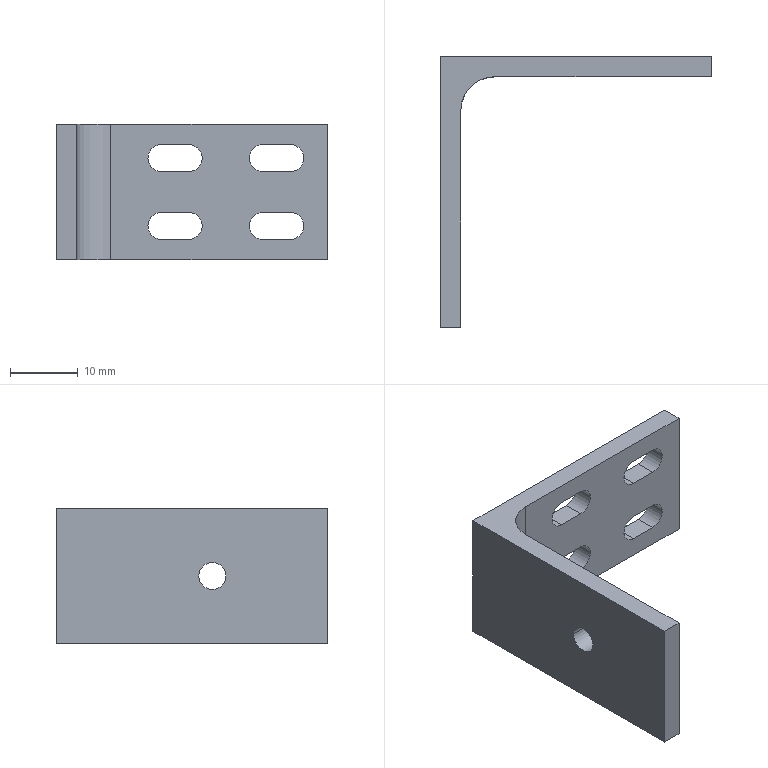Part | STEP file | L40 angle steel | 1 solid | 31 faces | box 40 x 40 x 20 mm | volume 4347 mm3 | plane 16 | cylinder 15 | commonest cylinder face diameters 4 x14 10 x1
STEP:
#1=CARTESIAN_POINT('',(3.,-21.,10.));
#2=VERTEX_POINT('',#1);
#3=CARTESIAN_POINT('',(3.,-25.,10.));
#4=VERTEX_POINT('',#3);
#5=CARTESIAN_POINT('',(3.,-23.,10.));
#6=DIRECTION('',(-1.,0.,0.));
#7=DIRECTION('',(0.,-1.,0.));
#8=AXIS2_PLACEMENT_3D('',#5,#6,#7);
#9=CIRCLE('',#8,2.);
#10=EDGE_CURVE('',#2,#4,#9,.T.);
#11=ORIENTED_EDGE('',*,*,#10,.F.);
#12=CARTESIAN_POINT('',(0.,-21.,10.));
#13=VERTEX_POINT('',#12);
#14=CARTESIAN_POINT('',(20.,-21.,10.));
#15=DIRECTION('',(-1.,0.,0.));
#16=VECTOR('',#15,1000.);
#17=LINE('',#14,#16);
#18=EDGE_CURVE('',#2,#13,#17,.T.);
#19=ORIENTED_EDGE('',*,*,#18,.T.);
#20=CARTESIAN_POINT('',(0.,-25.,10.));
#21=VERTEX_POINT('',#20);
#22=CARTESIAN_POINT('',(0.,-23.,10.));
#23=DIRECTION('',(-1.,0.,0.));
#24=DIRECTION('',(0.,-1.,0.));
#25=AXIS2_PLACEMENT_3D('',#22,#23,#24);
#26=CIRCLE('',#25,2.);
#27=EDGE_CURVE('',#13,#21,#26,.T.);
#28=ORIENTED_EDGE('',*,*,#27,.T.);
#29=CARTESIAN_POINT('',(20.,-25.,10.));
#30=DIRECTION('',(-1.,0.,0.));
#31=VECTOR('',#30,1000.);
#32=LINE('',#29,#31);
#33=EDGE_CURVE('',#4,#21,#32,.T.);
#34=ORIENTED_EDGE('',*,*,#33,.F.);
#35=EDGE_LOOP('',(#11,#19,#28,#34));
#36=FACE_OUTER_BOUND('',#35,.T.);
#37=CARTESIAN_POINT('',(20.,-23.,10.));
#38=DIRECTION('',(-1.,0.,0.));
#39=DIRECTION('',(0.,-1.,0.));
#40=AXIS2_PLACEMENT_3D('',#37,#38,#39);
#41=CYLINDRICAL_SURFACE('',#40,2.);
#42=ADVANCED_FACE('',(#36),#41,.F.);
#43=CARTESIAN_POINT('',(30.5,-3.,7.));
#44=VERTEX_POINT('',#43);
#45=CARTESIAN_POINT('',(28.5,-3.,5.));
#46=VERTEX_POINT('',#45);
#47=CARTESIAN_POINT('',(30.5,-3.,5.));
#48=DIRECTION('',(0.,-1.,0.));
#49=DIRECTION('',(-1.,0.,0.));
#50=AXIS2_PLACEMENT_3D('',#47,#48,#49);
#51=CIRCLE('',#50,2.);
#52=EDGE_CURVE('',#44,#46,#51,.T.);
#53=ORIENTED_EDGE('',*,*,#52,.T.);
#54=CARTESIAN_POINT('',(28.5,0.,5.));
#55=VERTEX_POINT('',#54);
#56=CARTESIAN_POINT('',(28.5,-20.,5.));
#57=DIRECTION('',(0.,1.,0.));
#58=VECTOR('',#57,1000.);
#59=LINE('',#56,#58);
#60=EDGE_CURVE('',#46,#55,#59,.T.);
#61=ORIENTED_EDGE('',*,*,#60,.T.);
#62=CARTESIAN_POINT('',(30.5,0.,7.));
#63=VERTEX_POINT('',#62);
#64=CARTESIAN_POINT('',(30.5,0.,5.));
#65=DIRECTION('',(0.,1.,0.));
#66=DIRECTION('',(-1.,0.,0.));
#67=AXIS2_PLACEMENT_3D('',#64,#65,#66);
#68=CIRCLE('',#67,2.);
#69=EDGE_CURVE('',#55,#63,#68,.T.);
#70=ORIENTED_EDGE('',*,*,#69,.T.);
#71=CARTESIAN_POINT('',(30.5,-20.,7.));
#72=DIRECTION('',(0.,-1.,0.));
#73=VECTOR('',#72,1000.);
#74=LINE('',#71,#73);
#75=EDGE_CURVE('',#63,#44,#74,.T.);
#76=ORIENTED_EDGE('',*,*,#75,.T.);
#77=EDGE_LOOP('',(#53,#61,#70,#76));
#78=FACE_OUTER_BOUND('',#77,.T.);
#79=CARTESIAN_POINT('',(30.5,-20.,5.));
#80=DIRECTION('',(0.,1.,0.));
#81=DIRECTION('',(-1.,0.,0.));
#82=AXIS2_PLACEMENT_3D('',#79,#80,#81);
#83=CYLINDRICAL_SURFACE('',#82,2.);
#84=ADVANCED_FACE('',(#78),#83,.F.);
#85=CARTESIAN_POINT('',(15.5,-3.,7.));
#86=VERTEX_POINT('',#85);
#87=CARTESIAN_POINT('',(13.5,-3.,5.));
#88=VERTEX_POINT('',#87);
#89=CARTESIAN_POINT('',(15.5,-3.,5.));
#90=DIRECTION('',(0.,-1.,0.));
#91=DIRECTION('',(-1.,0.,0.));
#92=AXIS2_PLACEMENT_3D('',#89,#90,#91);
#93=CIRCLE('',#92,2.);
#94=EDGE_CURVE('',#86,#88,#93,.T.);
#95=ORIENTED_EDGE('',*,*,#94,.T.);
#96=CARTESIAN_POINT('',(13.5,0.,5.));
#97=VERTEX_POINT('',#96);
#98=CARTESIAN_POINT('',(13.5,-20.,5.));
#99=DIRECTION('',(0.,1.,0.));
#100=VECTOR('',#99,1000.);
#101=LINE('',#98,#100);
#102=EDGE_CURVE('',#88,#97,#101,.T.);
#103=ORIENTED_EDGE('',*,*,#102,.T.);
#104=CARTESIAN_POINT('',(15.5,0.,7.));
#105=VERTEX_POINT('',#104);
#106=CARTESIAN_POINT('',(15.5,0.,5.));
#107=DIRECTION('',(0.,1.,0.));
#108=DIRECTION('',(-1.,0.,0.));
#109=AXIS2_PLACEMENT_3D('',#106,#107,#108);
#110=CIRCLE('',#109,2.);
#111=EDGE_CURVE('',#97,#105,#110,.T.);
#112=ORIENTED_EDGE('',*,*,#111,.T.);
#113=CARTESIAN_POINT('',(15.5,-20.,7.));
#114=DIRECTION('',(0.,-1.,0.));
#115=VECTOR('',#114,1000.);
#116=LINE('',#113,#115);
#117=EDGE_CURVE('',#105,#86,#116,.T.);
#118=ORIENTED_EDGE('',*,*,#117,.T.);
#119=EDGE_LOOP('',(#95,#103,#112,#118));
#120=FACE_OUTER_BOUND('',#119,.T.);
#121=CARTESIAN_POINT('',(15.5,-20.,5.));
#122=DIRECTION('',(0.,1.,0.));
#123=DIRECTION('',(-1.,0.,0.));
#124=AXIS2_PLACEMENT_3D('',#121,#122,#123);
#125=CYLINDRICAL_SURFACE('',#124,2.);
#126=ADVANCED_FACE('',(#120),#125,.F.);
#127=CARTESIAN_POINT('',(15.5,-3.,17.));
#128=VERTEX_POINT('',#127);
#129=CARTESIAN_POINT('',(13.5,-3.,15.));
#130=VERTEX_POINT('',#129);
#131=CARTESIAN_POINT('',(15.5,-3.,15.));
#132=DIRECTION('',(0.,-1.,0.));
#133=DIRECTION('',(-1.,0.,0.));
#134=AXIS2_PLACEMENT_3D('',#131,#132,#133);
#135=CIRCLE('',#134,2.);
#136=EDGE_CURVE('',#128,#130,#135,.T.);
#137=ORIENTED_EDGE('',*,*,#136,.T.);
#138=CARTESIAN_POINT('',(13.5,0.,15.));
#139=VERTEX_POINT('',#138);
#140=CARTESIAN_POINT('',(13.5,-20.,15.));
#141=DIRECTION('',(0.,1.,0.));
#142=VECTOR('',#141,1000.);
#143=LINE('',#140,#142);
#144=EDGE_CURVE('',#130,#139,#143,.T.);
#145=ORIENTED_EDGE('',*,*,#144,.T.);
#146=CARTESIAN_POINT('',(15.5,0.,17.));
#147=VERTEX_POINT('',#146);
#148=CARTESIAN_POINT('',(15.5,0.,15.));
#149=DIRECTION('',(0.,1.,0.));
#150=DIRECTION('',(-1.,0.,0.));
#151=AXIS2_PLACEMENT_3D('',#148,#149,#150);
#152=CIRCLE('',#151,2.);
#153=EDGE_CURVE('',#139,#147,#152,.T.);
#154=ORIENTED_EDGE('',*,*,#153,.T.);
#155=CARTESIAN_POINT('',(15.5,-20.,17.));
#156=DIRECTION('',(0.,-1.,0.));
#157=VECTOR('',#156,1000.);
#158=LINE('',#155,#157);
#159=EDGE_CURVE('',#147,#128,#158,.T.);
#160=ORIENTED_EDGE('',*,*,#159,.T.);
#161=EDGE_LOOP('',(#137,#145,#154,#160));
#162=FACE_OUTER_BOUND('',#161,.T.);
#163=CARTESIAN_POINT('',(15.5,-20.,15.));
#164=DIRECTION('',(0.,1.,0.));
#165=DIRECTION('',(-1.,0.,0.));
#166=AXIS2_PLACEMENT_3D('',#163,#164,#165);
#167=CYLINDRICAL_SURFACE('',#166,2.);
#168=ADVANCED_FACE('',(#162),#167,.F.);
#169=CARTESIAN_POINT('',(30.5,-3.,17.));
#170=VERTEX_POINT('',#169);
#171=CARTESIAN_POINT('',(28.5,-3.,15.));
#172=VERTEX_POINT('',#171);
#173=CARTESIAN_POINT('',(30.5,-3.,15.));
#174=DIRECTION('',(0.,-1.,0.));
#175=DIRECTION('',(-1.,0.,0.));
#176=AXIS2_PLACEMENT_3D('',#173,#174,#175);
#177=CIRCLE('',#176,2.);
#178=EDGE_CURVE('',#170,#172,#177,.T.);
#179=ORIENTED_EDGE('',*,*,#178,.T.);
#180=CARTESIAN_POINT('',(28.5,0.,15.));
#181=VERTEX_POINT('',#180);
#182=CARTESIAN_POINT('',(28.5,-20.,15.));
#183=DIRECTION('',(0.,1.,0.));
#184=VECTOR('',#183,1000.);
#185=LINE('',#182,#184);
#186=EDGE_CURVE('',#172,#181,#185,.T.);
#187=ORIENTED_EDGE('',*,*,#186,.T.);
#188=CARTESIAN_POINT('',(30.5,0.,17.));
#189=VERTEX_POINT('',#188);
#190=CARTESIAN_POINT('',(30.5,0.,15.));
#191=DIRECTION('',(0.,1.,0.));
#192=DIRECTION('',(-1.,0.,0.));
#193=AXIS2_PLACEMENT_3D('',#190,#191,#192);
#194=CIRCLE('',#193,2.);
#195=EDGE_CURVE('',#181,#189,#194,.T.);
#196=ORIENTED_EDGE('',*,*,#195,.T.);
#197=CARTESIAN_POINT('',(30.5,-20.,17.));
#198=DIRECTION('',(0.,-1.,0.));
#199=VECTOR('',#198,1000.);
#200=LINE('',#197,#199);
#201=EDGE_CURVE('',#189,#170,#200,.T.);
#202=ORIENTED_EDGE('',*,*,#201,.T.);
#203=EDGE_LOOP('',(#179,#187,#196,#202));
#204=FACE_OUTER_BOUND('',#203,.T.);
#205=CARTESIAN_POINT('',(30.5,-20.,15.));
#206=DIRECTION('',(0.,1.,0.));
#207=DIRECTION('',(-1.,0.,0.));
#208=AXIS2_PLACEMENT_3D('',#205,#206,#207);
#209=CYLINDRICAL_SURFACE('',#208,2.);
#210=ADVANCED_FACE('',(#204),#209,.F.);
#211=CARTESIAN_POINT('',(0.,-40.,20.));
#212=VERTEX_POINT('',#211);
#213=CARTESIAN_POINT('',(0.,-40.,0.));
#214=VERTEX_POINT('',#213);
#215=CARTESIAN_POINT('',(0.,-40.,20.));
#216=DIRECTION('',(0.,0.,-1.));
#217=VECTOR('',#216,1000.);
#218=LINE('',#215,#217);
#219=EDGE_CURVE('',#212,#214,#218,.T.);
#220=ORIENTED_EDGE('',*,*,#219,.F.);
#221=CARTESIAN_POINT('',(0.,0.,20.));
#222=VERTEX_POINT('',#221);
#223=CARTESIAN_POINT('',(0.,0.,20.));
#224=DIRECTION('',(0.,-1.,0.));
#225=VECTOR('',#224,1000.);
#226=LINE('',#223,#225);
#227=EDGE_CURVE('',#222,#212,#226,.T.);
#228=ORIENTED_EDGE('',*,*,#227,.F.);
#229=CARTESIAN_POINT('',(0.,0.,0.));
#230=VERTEX_POINT('',#229);
#231=CARTESIAN_POINT('',(0.,0.,20.));
#232=DIRECTION('',(0.,0.,1.));
#233=VECTOR('',#232,1000.);
#234=LINE('',#231,#233);
#235=EDGE_CURVE('',#230,#222,#234,.T.);
#236=ORIENTED_EDGE('',*,*,#235,.F.);
#237=CARTESIAN_POINT('',(0.,0.,0.));
#238=DIRECTION('',(0.,1.,0.));
#239=VECTOR('',#238,1000.);
#240=LINE('',#237,#239);
#241=EDGE_CURVE('',#214,#230,#240,.T.);
#242=ORIENTED_EDGE('',*,*,#241,.F.);
#243=EDGE_LOOP('',(#220,#228,#236,#242));
#244=FACE_OUTER_BOUND('',#243,.T.);
#245=CARTESIAN_POINT('',(0.,-23.,10.));
#246=DIRECTION('',(-1.,0.,0.));
#247=DIRECTION('',(0.,-1.,0.));
#248=AXIS2_PLACEMENT_3D('',#245,#246,#247);
#249=CIRCLE('',#248,2.);
#250=EDGE_CURVE('',#21,#13,#249,.T.);
#251=ORIENTED_EDGE('',*,*,#250,.F.);
#252=ORIENTED_EDGE('',*,*,#27,.F.);
#253=EDGE_LOOP('',(#251,#252));
#254=FACE_BOUND('',#253,.T.);
#255=CARTESIAN_POINT('',(0.,0.,20.));
#256=DIRECTION('',(1.,0.,0.));
#257=DIRECTION('',(0.,1.,0.));
#258=AXIS2_PLACEMENT_3D('',#255,#256,#257);
#259=PLANE('',#258);
#260=ADVANCED_FACE('',(#244,#254),#259,.F.);
#261=ORIENTED_EDGE('',*,*,#241,.T.);
#262=CARTESIAN_POINT('',(40.,0.,0.));
#263=VERTEX_POINT('',#262);
#264=CARTESIAN_POINT('',(8.,0.,0.));
#265=DIRECTION('',(1.,0.,0.));
#266=VECTOR('',#265,1000.);
#267=LINE('',#264,#266);
#268=EDGE_CURVE('',#230,#263,#267,.T.);
#269=ORIENTED_EDGE('',*,*,#268,.T.);
#270=CARTESIAN_POINT('',(40.,-3.,0.));
#271=VERTEX_POINT('',#270);
#272=CARTESIAN_POINT('',(40.,-8.,0.));
#273=DIRECTION('',(0.,-1.,0.));
#274=VECTOR('',#273,1000.);
#275=LINE('',#272,#274);
#276=EDGE_CURVE('',#263,#271,#275,.T.);
#277=ORIENTED_EDGE('',*,*,#276,.T.);
#278=CARTESIAN_POINT('',(8.,-3.,0.));
#279=VERTEX_POINT('',#278);
#280=CARTESIAN_POINT('',(8.,-3.,0.));
#281=DIRECTION('',(-1.,0.,0.));
#282=VECTOR('',#281,1000.);
#283=LINE('',#280,#282);
#284=EDGE_CURVE('',#271,#279,#283,.T.);
#285=ORIENTED_EDGE('',*,*,#284,.T.);
#286=CARTESIAN_POINT('',(3.,-8.,0.));
#287=VERTEX_POINT('',#286);
#288=CARTESIAN_POINT('',(8.,-8.,0.));
#289=DIRECTION('',(0.,0.,1.));
#290=DIRECTION('',(-1.,0.,0.));
#291=AXIS2_PLACEMENT_3D('',#288,#289,#290);
#292=CIRCLE('',#291,5.);
#293=EDGE_CURVE('',#279,#287,#292,.T.);
#294=ORIENTED_EDGE('',*,*,#293,.T.);
#295=CARTESIAN_POINT('',(3.,-40.,0.));
#296=VERTEX_POINT('',#295);
#297=CARTESIAN_POINT('',(3.,-8.,0.));
#298=DIRECTION('',(0.,-1.,0.));
#299=VECTOR('',#298,1000.);
#300=LINE('',#297,#299);
#301=EDGE_CURVE('',#287,#296,#300,.T.);
#302=ORIENTED_EDGE('',*,*,#301,.T.);
#303=CARTESIAN_POINT('',(8.,-40.,0.));
#304=DIRECTION('',(-1.,0.,0.));
#305=VECTOR('',#304,1000.);
#306=LINE('',#303,#305);
#307=EDGE_CURVE('',#296,#214,#306,.T.);
#308=ORIENTED_EDGE('',*,*,#307,.T.);
#309=EDGE_LOOP('',(#261,#269,#277,#285,#294,#302,#308));
#310=FACE_OUTER_BOUND('',#309,.T.);
#311=CARTESIAN_POINT('',(8.,-8.,0.));
#312=DIRECTION('',(0.,0.,-1.));
#313=DIRECTION('',(-1.,0.,0.));
#314=AXIS2_PLACEMENT_3D('',#311,#312,#313);
#315=PLANE('',#314);
#316=ADVANCED_FACE('',(#310),#315,.T.);
#317=CARTESIAN_POINT('',(3.,-40.,20.));
#318=VERTEX_POINT('',#317);
#319=CARTESIAN_POINT('',(3.,-40.,20.));
#320=DIRECTION('',(0.,0.,-1.));
#321=VECTOR('',#320,1000.);
#322=LINE('',#319,#321);
#323=EDGE_CURVE('',#318,#296,#322,.T.);
#324=ORIENTED_EDGE('',*,*,#323,.F.);
#325=CARTESIAN_POINT('',(3.,-40.,20.));
#326=DIRECTION('',(1.,0.,0.));
#327=VECTOR('',#326,1000.);
#328=LINE('',#325,#327);
#329=EDGE_CURVE('',#212,#318,#328,.T.);
#330=ORIENTED_EDGE('',*,*,#329,.F.);
#331=ORIENTED_EDGE('',*,*,#219,.T.);
#332=ORIENTED_EDGE('',*,*,#307,.F.);
#333=EDGE_LOOP('',(#324,#330,#331,#332));
#334=FACE_OUTER_BOUND('',#333,.T.);
#335=CARTESIAN_POINT('',(3.,-40.,20.));
#336=DIRECTION('',(0.,1.,0.));
#337=DIRECTION('',(0.,0.,1.));
#338=AXIS2_PLACEMENT_3D('',#335,#336,#337);
#339=PLANE('',#338);
#340=ADVANCED_FACE('',(#334),#339,.F.);
#341=CARTESIAN_POINT('',(40.,0.,20.));
#342=VERTEX_POINT('',#341);
#343=CARTESIAN_POINT('',(8.,0.,20.));
#344=DIRECTION('',(1.,0.,0.));
#345=VECTOR('',#344,1000.);
#346=LINE('',#343,#345);
#347=EDGE_CURVE('',#222,#342,#346,.T.);
#348=ORIENTED_EDGE('',*,*,#347,.F.);
#349=ORIENTED_EDGE('',*,*,#227,.T.);
#350=ORIENTED_EDGE('',*,*,#329,.T.);
#351=CARTESIAN_POINT('',(3.,-8.,20.));
#352=VERTEX_POINT('',#351);
#353=CARTESIAN_POINT('',(3.,-8.,20.));
#354=DIRECTION('',(0.,-1.,0.));
#355=VECTOR('',#354,1000.);
#356=LINE('',#353,#355);
#357=EDGE_CURVE('',#352,#318,#356,.T.);
#358=ORIENTED_EDGE('',*,*,#357,.F.);
#359=CARTESIAN_POINT('',(8.,-3.,20.));
#360=VERTEX_POINT('',#359);
#361=CARTESIAN_POINT('',(8.,-8.,20.));
#362=DIRECTION('',(0.,0.,1.));
#363=DIRECTION('',(-1.,0.,0.));
#364=AXIS2_PLACEMENT_3D('',#361,#362,#363);
#365=CIRCLE('',#364,5.);
#366=EDGE_CURVE('',#360,#352,#365,.T.);
#367=ORIENTED_EDGE('',*,*,#366,.F.);
#368=CARTESIAN_POINT('',(40.,-3.,20.));
#369=VERTEX_POINT('',#368);
#370=CARTESIAN_POINT('',(8.,-3.,20.));
#371=DIRECTION('',(-1.,0.,0.));
#372=VECTOR('',#371,1000.);
#373=LINE('',#370,#372);
#374=EDGE_CURVE('',#369,#360,#373,.T.);
#375=ORIENTED_EDGE('',*,*,#374,.F.);
#376=CARTESIAN_POINT('',(40.,-8.,20.));
#377=DIRECTION('',(0.,-1.,0.));
#378=VECTOR('',#377,1000.);
#379=LINE('',#376,#378);
#380=EDGE_CURVE('',#342,#369,#379,.T.);
#381=ORIENTED_EDGE('',*,*,#380,.F.);
#382=EDGE_LOOP('',(#348,#349,#350,#358,#367,#375,#381));
#383=FACE_OUTER_BOUND('',#382,.T.);
#384=CARTESIAN_POINT('',(8.,-8.,20.));
#385=DIRECTION('',(0.,0.,-1.));
#386=DIRECTION('',(-1.,0.,0.));
#387=AXIS2_PLACEMENT_3D('',#384,#385,#386);
#388=PLANE('',#387);
#389=ADVANCED_FACE('',(#383),#388,.F.);
#390=ORIENTED_EDGE('',*,*,#235,.T.);
#391=ORIENTED_EDGE('',*,*,#347,.T.);
#392=CARTESIAN_POINT('',(40.,0.,20.));
#393=DIRECTION('',(0.,0.,1.));
#394=VECTOR('',#393,1000.);
#395=LINE('',#392,#394);
#396=EDGE_CURVE('',#263,#342,#395,.T.);
#397=ORIENTED_EDGE('',*,*,#396,.F.);
#398=ORIENTED_EDGE('',*,*,#268,.F.);
#399=EDGE_LOOP('',(#390,#391,#397,#398));
#400=FACE_OUTER_BOUND('',#399,.T.);
#401=CARTESIAN_POINT('',(30.5,0.,3.));
#402=VERTEX_POINT('',#401);
#403=CARTESIAN_POINT('',(30.5,0.,5.));
#404=DIRECTION('',(0.,1.,0.));
#405=DIRECTION('',(-1.,0.,0.));
#406=AXIS2_PLACEMENT_3D('',#403,#404,#405);
#407=CIRCLE('',#406,2.);
#408=EDGE_CURVE('',#402,#55,#407,.T.);
#409=ORIENTED_EDGE('',*,*,#408,.F.);
#410=CARTESIAN_POINT('',(34.5,0.,3.));
#411=VERTEX_POINT('',#410);
#412=CARTESIAN_POINT('',(40.,0.,3.));
#413=DIRECTION('',(-1.,0.,0.));
#414=VECTOR('',#413,1000.);
#415=LINE('',#412,#414);
#416=EDGE_CURVE('',#411,#402,#415,.T.);
#417=ORIENTED_EDGE('',*,*,#416,.F.);
#418=CARTESIAN_POINT('',(34.5,0.,7.));
#419=VERTEX_POINT('',#418);
#420=CARTESIAN_POINT('',(34.5,0.,5.));
#421=DIRECTION('',(0.,1.,0.));
#422=DIRECTION('',(-1.,0.,0.));
#423=AXIS2_PLACEMENT_3D('',#420,#421,#422);
#424=CIRCLE('',#423,2.);
#425=EDGE_CURVE('',#419,#411,#424,.T.);
#426=ORIENTED_EDGE('',*,*,#425,.F.);
#427=CARTESIAN_POINT('',(40.,0.,7.));
#428=DIRECTION('',(1.,0.,0.));
#429=VECTOR('',#428,1000.);
#430=LINE('',#427,#429);
#431=EDGE_CURVE('',#63,#419,#430,.T.);
#432=ORIENTED_EDGE('',*,*,#431,.F.);
#433=ORIENTED_EDGE('',*,*,#69,.F.);
#434=EDGE_LOOP('',(#409,#417,#426,#432,#433));
#435=FACE_BOUND('',#434,.T.);
#436=CARTESIAN_POINT('',(15.5,0.,3.));
#437=VERTEX_POINT('',#436);
#438=CARTESIAN_POINT('',(15.5,0.,5.));
#439=DIRECTION('',(0.,1.,0.));
#440=DIRECTION('',(-1.,0.,0.));
#441=AXIS2_PLACEMENT_3D('',#438,#439,#440);
#442=CIRCLE('',#441,2.);
#443=EDGE_CURVE('',#437,#97,#442,.T.);
#444=ORIENTED_EDGE('',*,*,#443,.F.);
#445=CARTESIAN_POINT('',(19.5,0.,3.));
#446=VERTEX_POINT('',#445);
#447=CARTESIAN_POINT('',(40.,0.,3.));
#448=DIRECTION('',(-1.,0.,0.));
#449=VECTOR('',#448,1000.);
#450=LINE('',#447,#449);
#451=EDGE_CURVE('',#446,#437,#450,.T.);
#452=ORIENTED_EDGE('',*,*,#451,.F.);
#453=CARTESIAN_POINT('',(19.5,0.,7.));
#454=VERTEX_POINT('',#453);
#455=CARTESIAN_POINT('',(19.5,0.,5.));
#456=DIRECTION('',(0.,1.,0.));
#457=DIRECTION('',(-1.,0.,0.));
#458=AXIS2_PLACEMENT_3D('',#455,#456,#457);
#459=CIRCLE('',#458,2.);
#460=EDGE_CURVE('',#454,#446,#459,.T.);
#461=ORIENTED_EDGE('',*,*,#460,.F.);
#462=CARTESIAN_POINT('',(40.,0.,7.));
#463=DIRECTION('',(1.,0.,0.));
#464=VECTOR('',#463,1000.);
#465=LINE('',#462,#464);
#466=EDGE_CURVE('',#105,#454,#465,.T.);
#467=ORIENTED_EDGE('',*,*,#466,.F.);
#468=ORIENTED_EDGE('',*,*,#111,.F.);
#469=EDGE_LOOP('',(#444,#452,#461,#467,#468));
#470=FACE_BOUND('',#469,.T.);
#471=CARTESIAN_POINT('',(15.5,0.,13.));
#472=VERTEX_POINT('',#471);
#473=CARTESIAN_POINT('',(15.5,0.,15.));
#474=DIRECTION('',(0.,1.,0.));
#475=DIRECTION('',(-1.,0.,0.));
#476=AXIS2_PLACEMENT_3D('',#473,#474,#475);
#477=CIRCLE('',#476,2.);
#478=EDGE_CURVE('',#472,#139,#477,.T.);
#479=ORIENTED_EDGE('',*,*,#478,.F.);
#480=CARTESIAN_POINT('',(19.5,0.,13.));
#481=VERTEX_POINT('',#480);
#482=CARTESIAN_POINT('',(40.,0.,13.));
#483=DIRECTION('',(-1.,0.,0.));
#484=VECTOR('',#483,1000.);
#485=LINE('',#482,#484);
#486=EDGE_CURVE('',#481,#472,#485,.T.);
#487=ORIENTED_EDGE('',*,*,#486,.F.);
#488=CARTESIAN_POINT('',(19.5,0.,17.));
#489=VERTEX_POINT('',#488);
#490=CARTESIAN_POINT('',(19.5,0.,15.));
#491=DIRECTION('',(0.,1.,0.));
#492=DIRECTION('',(-1.,0.,0.));
#493=AXIS2_PLACEMENT_3D('',#490,#491,#492);
#494=CIRCLE('',#493,2.);
#495=EDGE_CURVE('',#489,#481,#494,.T.);
#496=ORIENTED_EDGE('',*,*,#495,.F.);
#497=CARTESIAN_POINT('',(40.,0.,17.));
#498=DIRECTION('',(1.,0.,0.));
#499=VECTOR('',#498,1000.);
#500=LINE('',#497,#499);
#501=EDGE_CURVE('',#147,#489,#500,.T.);
#502=ORIENTED_EDGE('',*,*,#501,.F.);
#503=ORIENTED_EDGE('',*,*,#153,.F.);
#504=EDGE_LOOP('',(#479,#487,#496,#502,#503));
#505=FACE_BOUND('',#504,.T.);
#506=CARTESIAN_POINT('',(30.5,0.,13.));
#507=VERTEX_POINT('',#506);
#508=CARTESIAN_POINT('',(30.5,0.,15.));
#509=DIRECTION('',(0.,1.,0.));
#510=DIRECTION('',(-1.,0.,0.));
#511=AXIS2_PLACEMENT_3D('',#508,#509,#510);
#512=CIRCLE('',#511,2.);
#513=EDGE_CURVE('',#507,#181,#512,.T.);
#514=ORIENTED_EDGE('',*,*,#513,.F.);
#515=CARTESIAN_POINT('',(34.5,0.,13.));
#516=VERTEX_POINT('',#515);
#517=CARTESIAN_POINT('',(40.,0.,13.));
#518=DIRECTION('',(-1.,0.,0.));
#519=VECTOR('',#518,1000.);
#520=LINE('',#517,#519);
#521=EDGE_CURVE('',#516,#507,#520,.T.);
#522=ORIENTED_EDGE('',*,*,#521,.F.);
#523=CARTESIAN_POINT('',(34.5,0.,17.));
#524=VERTEX_POINT('',#523);
#525=CARTESIAN_POINT('',(34.5,0.,15.));
#526=DIRECTION('',(0.,1.,0.));
#527=DIRECTION('',(-1.,0.,0.));
#528=AXIS2_PLACEMENT_3D('',#525,#526,#527);
#529=CIRCLE('',#528,2.);
#530=EDGE_CURVE('',#524,#516,#529,.T.);
#531=ORIENTED_EDGE('',*,*,#530,.F.);
#532=CARTESIAN_POINT('',(40.,0.,17.));
#533=DIRECTION('',(1.,0.,0.));
#534=VECTOR('',#533,1000.);
#535=LINE('',#532,#534);
#536=EDGE_CURVE('',#189,#524,#535,.T.);
#537=ORIENTED_EDGE('',*,*,#536,.F.);
#538=ORIENTED_EDGE('',*,*,#195,.F.);
#539=EDGE_LOOP('',(#514,#522,#531,#537,#538));
#540=FACE_BOUND('',#539,.T.);
#541=CARTESIAN_POINT('',(40.,0.,20.));
#542=DIRECTION('',(0.,-1.,0.));
#543=DIRECTION('',(1.,0.,0.));
#544=AXIS2_PLACEMENT_3D('',#541,#542,#543);
#545=PLANE('',#544);
#546=ADVANCED_FACE('',(#400,#435,#470,#505,#540),#545,.F.);
#547=ORIENTED_EDGE('',*,*,#18,.F.);
#548=CARTESIAN_POINT('',(3.,-23.,10.));
#549=DIRECTION('',(-1.,0.,0.));
#550=DIRECTION('',(0.,-1.,0.));
#551=AXIS2_PLACEMENT_3D('',#548,#549,#550);
#552=CIRCLE('',#551,2.);
#553=EDGE_CURVE('',#4,#2,#552,.T.);
#554=ORIENTED_EDGE('',*,*,#553,.F.);
#555=ORIENTED_EDGE('',*,*,#33,.T.);
#556=ORIENTED_EDGE('',*,*,#250,.T.);
#557=EDGE_LOOP('',(#547,#554,#555,#556));
#558=FACE_OUTER_BOUND('',#557,.T.);
#559=CARTESIAN_POINT('',(20.,-23.,10.));
#560=DIRECTION('',(-1.,0.,0.));
#561=DIRECTION('',(0.,-1.,0.));
#562=AXIS2_PLACEMENT_3D('',#559,#560,#561);
#563=CYLINDRICAL_SURFACE('',#562,2.);
#564=ADVANCED_FACE('',(#558),#563,.F.);
#565=CARTESIAN_POINT('',(3.,-8.,20.));
#566=DIRECTION('',(0.,0.,-1.));
#567=VECTOR('',#566,1000.);
#568=LINE('',#565,#567);
#569=EDGE_CURVE('',#352,#287,#568,.T.);
#570=ORIENTED_EDGE('',*,*,#569,.F.);
#571=ORIENTED_EDGE('',*,*,#357,.T.);
#572=ORIENTED_EDGE('',*,*,#323,.T.);
#573=ORIENTED_EDGE('',*,*,#301,.F.);
#574=EDGE_LOOP('',(#570,#571,#572,#573));
#575=FACE_OUTER_BOUND('',#574,.T.);
#576=ORIENTED_EDGE('',*,*,#553,.T.);
#577=ORIENTED_EDGE('',*,*,#10,.T.);
#578=EDGE_LOOP('',(#576,#577));
#579=FACE_BOUND('',#578,.T.);
#580=CARTESIAN_POINT('',(3.,-8.,20.));
#581=DIRECTION('',(-1.,0.,0.));
#582=DIRECTION('',(0.,-1.,0.));
#583=AXIS2_PLACEMENT_3D('',#580,#581,#582);
#584=PLANE('',#583);
#585=ADVANCED_FACE('',(#575,#579),#584,.F.);
#586=CARTESIAN_POINT('',(8.,-3.,20.));
#587=DIRECTION('',(0.,0.,-1.));
#588=VECTOR('',#587,1000.);
#589=LINE('',#586,#588);
#590=EDGE_CURVE('',#360,#279,#589,.T.);
#591=ORIENTED_EDGE('',*,*,#590,.F.);
#592=ORIENTED_EDGE('',*,*,#366,.T.);
#593=ORIENTED_EDGE('',*,*,#569,.T.);
#594=ORIENTED_EDGE('',*,*,#293,.F.);
#595=EDGE_LOOP('',(#591,#592,#593,#594));
#596=FACE_OUTER_BOUND('',#595,.T.);
#597=CARTESIAN_POINT('',(8.,-8.,20.));
#598=DIRECTION('',(0.,0.,-1.));
#599=DIRECTION('',(-1.,0.,0.));
#600=AXIS2_PLACEMENT_3D('',#597,#598,#599);
#601=CYLINDRICAL_SURFACE('',#600,5.);
#602=ADVANCED_FACE('',(#596),#601,.F.);
#603=CARTESIAN_POINT('',(40.,-3.,20.));
#604=DIRECTION('',(0.,0.,-1.));
#605=VECTOR('',#604,1000.);
#606=LINE('',#603,#605);
#607=EDGE_CURVE('',#369,#271,#606,.T.);
#608=ORIENTED_EDGE('',*,*,#607,.F.);
#609=ORIENTED_EDGE('',*,*,#374,.T.);
#610=ORIENTED_EDGE('',*,*,#590,.T.);
#611=ORIENTED_EDGE('',*,*,#284,.F.);
#612=EDGE_LOOP('',(#608,#609,#610,#611));
#613=FACE_OUTER_BOUND('',#612,.T.);
#614=ORIENTED_EDGE('',*,*,#52,.F.);
#615=CARTESIAN_POINT('',(34.5,-3.,7.));
#616=VERTEX_POINT('',#615);
#617=CARTESIAN_POINT('',(40.,-3.,7.));
#618=DIRECTION('',(-1.,0.,0.));
#619=VECTOR('',#618,1000.);
#620=LINE('',#617,#619);
#621=EDGE_CURVE('',#616,#44,#620,.T.);
#622=ORIENTED_EDGE('',*,*,#621,.F.);
#623=CARTESIAN_POINT('',(34.5,-3.,3.));
#624=VERTEX_POINT('',#623);
#625=CARTESIAN_POINT('',(34.5,-3.,5.));
#626=DIRECTION('',(0.,-1.,0.));
#627=DIRECTION('',(-1.,0.,0.));
#628=AXIS2_PLACEMENT_3D('',#625,#626,#627);
#629=CIRCLE('',#628,2.);
#630=EDGE_CURVE('',#624,#616,#629,.T.);
#631=ORIENTED_EDGE('',*,*,#630,.F.);
#632=CARTESIAN_POINT('',(30.5,-3.,3.));
#633=VERTEX_POINT('',#632);
#634=CARTESIAN_POINT('',(40.,-3.,3.));
#635=DIRECTION('',(1.,0.,0.));
#636=VECTOR('',#635,1000.);
#637=LINE('',#634,#636);
#638=EDGE_CURVE('',#633,#624,#637,.T.);
#639=ORIENTED_EDGE('',*,*,#638,.F.);
#640=CARTESIAN_POINT('',(30.5,-3.,5.));
#641=DIRECTION('',(0.,-1.,0.));
#642=DIRECTION('',(-1.,0.,0.));
#643=AXIS2_PLACEMENT_3D('',#640,#641,#642);
#644=CIRCLE('',#643,2.);
#645=EDGE_CURVE('',#46,#633,#644,.T.);
#646=ORIENTED_EDGE('',*,*,#645,.F.);
#647=EDGE_LOOP('',(#614,#622,#631,#639,#646));
#648=FACE_BOUND('',#647,.T.);
#649=ORIENTED_EDGE('',*,*,#94,.F.);
#650=CARTESIAN_POINT('',(19.5,-3.,7.));
#651=VERTEX_POINT('',#650);
#652=CARTESIAN_POINT('',(40.,-3.,7.));
#653=DIRECTION('',(-1.,0.,0.));
#654=VECTOR('',#653,1000.);
#655=LINE('',#652,#654);
#656=EDGE_CURVE('',#651,#86,#655,.T.);
#657=ORIENTED_EDGE('',*,*,#656,.F.);
#658=CARTESIAN_POINT('',(19.5,-3.,3.));
#659=VERTEX_POINT('',#658);
#660=CARTESIAN_POINT('',(19.5,-3.,5.));
#661=DIRECTION('',(0.,-1.,0.));
#662=DIRECTION('',(-1.,0.,0.));
#663=AXIS2_PLACEMENT_3D('',#660,#661,#662);
#664=CIRCLE('',#663,2.);
#665=EDGE_CURVE('',#659,#651,#664,.T.);
#666=ORIENTED_EDGE('',*,*,#665,.F.);
#667=CARTESIAN_POINT('',(15.5,-3.,3.));
#668=VERTEX_POINT('',#667);
#669=CARTESIAN_POINT('',(40.,-3.,3.));
#670=DIRECTION('',(1.,0.,0.));
#671=VECTOR('',#670,1000.);
#672=LINE('',#669,#671);
#673=EDGE_CURVE('',#668,#659,#672,.T.);
#674=ORIENTED_EDGE('',*,*,#673,.F.);
#675=CARTESIAN_POINT('',(15.5,-3.,5.));
#676=DIRECTION('',(0.,-1.,0.));
#677=DIRECTION('',(-1.,0.,0.));
#678=AXIS2_PLACEMENT_3D('',#675,#676,#677);
#679=CIRCLE('',#678,2.);
#680=EDGE_CURVE('',#88,#668,#679,.T.);
#681=ORIENTED_EDGE('',*,*,#680,.F.);
#682=EDGE_LOOP('',(#649,#657,#666,#674,#681));
#683=FACE_BOUND('',#682,.T.);
#684=ORIENTED_EDGE('',*,*,#136,.F.);
#685=CARTESIAN_POINT('',(19.5,-3.,17.));
#686=VERTEX_POINT('',#685);
#687=CARTESIAN_POINT('',(40.,-3.,17.));
#688=DIRECTION('',(-1.,0.,0.));
#689=VECTOR('',#688,1000.);
#690=LINE('',#687,#689);
#691=EDGE_CURVE('',#686,#128,#690,.T.);
#692=ORIENTED_EDGE('',*,*,#691,.F.);
#693=CARTESIAN_POINT('',(19.5,-3.,13.));
#694=VERTEX_POINT('',#693);
#695=CARTESIAN_POINT('',(19.5,-3.,15.));
#696=DIRECTION('',(0.,-1.,0.));
#697=DIRECTION('',(-1.,0.,0.));
#698=AXIS2_PLACEMENT_3D('',#695,#696,#697);
#699=CIRCLE('',#698,2.);
#700=EDGE_CURVE('',#694,#686,#699,.T.);
#701=ORIENTED_EDGE('',*,*,#700,.F.);
#702=CARTESIAN_POINT('',(15.5,-3.,13.));
#703=VERTEX_POINT('',#702);
#704=CARTESIAN_POINT('',(40.,-3.,13.));
#705=DIRECTION('',(1.,0.,0.));
#706=VECTOR('',#705,1000.);
#707=LINE('',#704,#706);
#708=EDGE_CURVE('',#703,#694,#707,.T.);
#709=ORIENTED_EDGE('',*,*,#708,.F.);
#710=CARTESIAN_POINT('',(15.5,-3.,15.));
#711=DIRECTION('',(0.,-1.,0.));
#712=DIRECTION('',(-1.,0.,0.));
#713=AXIS2_PLACEMENT_3D('',#710,#711,#712);
#714=CIRCLE('',#713,2.);
#715=EDGE_CURVE('',#130,#703,#714,.T.);
#716=ORIENTED_EDGE('',*,*,#715,.F.);
#717=EDGE_LOOP('',(#684,#692,#701,#709,#716));
#718=FACE_BOUND('',#717,.T.);
#719=ORIENTED_EDGE('',*,*,#178,.F.);
#720=CARTESIAN_POINT('',(34.5,-3.,17.));
#721=VERTEX_POINT('',#720);
#722=CARTESIAN_POINT('',(40.,-3.,17.));
#723=DIRECTION('',(-1.,0.,0.));
#724=VECTOR('',#723,1000.);
#725=LINE('',#722,#724);
#726=EDGE_CURVE('',#721,#170,#725,.T.);
#727=ORIENTED_EDGE('',*,*,#726,.F.);
#728=CARTESIAN_POINT('',(34.5,-3.,13.));
#729=VERTEX_POINT('',#728);
#730=CARTESIAN_POINT('',(34.5,-3.,15.));
#731=DIRECTION('',(0.,-1.,0.));
#732=DIRECTION('',(-1.,0.,0.));
#733=AXIS2_PLACEMENT_3D('',#730,#731,#732);
#734=CIRCLE('',#733,2.);
#735=EDGE_CURVE('',#729,#721,#734,.T.);
#736=ORIENTED_EDGE('',*,*,#735,.F.);
#737=CARTESIAN_POINT('',(30.5,-3.,13.));
#738=VERTEX_POINT('',#737);
#739=CARTESIAN_POINT('',(40.,-3.,13.));
#740=DIRECTION('',(1.,0.,0.));
#741=VECTOR('',#740,1000.);
#742=LINE('',#739,#741);
#743=EDGE_CURVE('',#738,#729,#742,.T.);
#744=ORIENTED_EDGE('',*,*,#743,.F.);
#745=CARTESIAN_POINT('',(30.5,-3.,15.));
#746=DIRECTION('',(0.,-1.,0.));
#747=DIRECTION('',(-1.,0.,0.));
#748=AXIS2_PLACEMENT_3D('',#745,#746,#747);
#749=CIRCLE('',#748,2.);
#750=EDGE_CURVE('',#172,#738,#749,.T.);
#751=ORIENTED_EDGE('',*,*,#750,.F.);
#752=EDGE_LOOP('',(#719,#727,#736,#744,#751));
#753=FACE_BOUND('',#752,.T.);
#754=CARTESIAN_POINT('',(40.,-3.,20.));
#755=DIRECTION('',(0.,1.,0.));
#756=DIRECTION('',(-1.,0.,0.));
#757=AXIS2_PLACEMENT_3D('',#754,#755,#756);
#758=PLANE('',#757);
#759=ADVANCED_FACE('',(#613,#648,#683,#718,#753),#758,.F.);
#760=ORIENTED_EDGE('',*,*,#396,.T.);
#761=ORIENTED_EDGE('',*,*,#380,.T.);
#762=ORIENTED_EDGE('',*,*,#607,.T.);
#763=ORIENTED_EDGE('',*,*,#276,.F.);
#764=EDGE_LOOP('',(#760,#761,#762,#763));
#765=FACE_OUTER_BOUND('',#764,.T.);
#766=CARTESIAN_POINT('',(40.,0.,20.));
#767=DIRECTION('',(-1.,0.,0.));
#768=DIRECTION('',(0.,0.,1.));
#769=AXIS2_PLACEMENT_3D('',#766,#767,#768);
#770=PLANE('',#769);
#771=ADVANCED_FACE('',(#765),#770,.F.);
#772=ORIENTED_EDGE('',*,*,#431,.T.);
#773=CARTESIAN_POINT('',(34.5,-20.,7.));
#774=DIRECTION('',(0.,1.,0.));
#775=VECTOR('',#774,1000.);
#776=LINE('',#773,#775);
#777=EDGE_CURVE('',#616,#419,#776,.T.);
#778=ORIENTED_EDGE('',*,*,#777,.F.);
#779=ORIENTED_EDGE('',*,*,#621,.T.);
#780=ORIENTED_EDGE('',*,*,#75,.F.);
#781=EDGE_LOOP('',(#772,#778,#779,#780));
#782=FACE_OUTER_BOUND('',#781,.T.);
#783=CARTESIAN_POINT('',(30.5,-20.,7.));
#784=DIRECTION('',(0.,0.,1.));
#785=DIRECTION('',(1.,0.,0.));
#786=AXIS2_PLACEMENT_3D('',#783,#784,#785);
#787=PLANE('',#786);
#788=ADVANCED_FACE('',(#782),#787,.F.);
#789=ORIENTED_EDGE('',*,*,#60,.F.);
#790=ORIENTED_EDGE('',*,*,#645,.T.);
#791=CARTESIAN_POINT('',(30.5,-20.,3.));
#792=DIRECTION('',(0.,-1.,0.));
#793=VECTOR('',#792,1000.);
#794=LINE('',#791,#793);
#795=EDGE_CURVE('',#402,#633,#794,.T.);
#796=ORIENTED_EDGE('',*,*,#795,.F.);
#797=ORIENTED_EDGE('',*,*,#408,.T.);
#798=EDGE_LOOP('',(#789,#790,#796,#797));
#799=FACE_OUTER_BOUND('',#798,.T.);
#800=CARTESIAN_POINT('',(30.5,-20.,5.));
#801=DIRECTION('',(0.,1.,0.));
#802=DIRECTION('',(-1.,0.,0.));
#803=AXIS2_PLACEMENT_3D('',#800,#801,#802);
#804=CYLINDRICAL_SURFACE('',#803,2.);
#805=ADVANCED_FACE('',(#799),#804,.F.);
#806=ORIENTED_EDGE('',*,*,#416,.T.);
#807=ORIENTED_EDGE('',*,*,#795,.T.);
#808=ORIENTED_EDGE('',*,*,#638,.T.);
#809=CARTESIAN_POINT('',(34.5,-20.,3.));
#810=DIRECTION('',(0.,-1.,0.));
#811=VECTOR('',#810,1000.);
#812=LINE('',#809,#811);
#813=EDGE_CURVE('',#411,#624,#812,.T.);
#814=ORIENTED_EDGE('',*,*,#813,.F.);
#815=EDGE_LOOP('',(#806,#807,#808,#814));
#816=FACE_OUTER_BOUND('',#815,.T.);
#817=CARTESIAN_POINT('',(30.5,-20.,3.));
#818=DIRECTION('',(0.,0.,-1.));
#819=DIRECTION('',(-1.,0.,0.));
#820=AXIS2_PLACEMENT_3D('',#817,#818,#819);
#821=PLANE('',#820);
#822=ADVANCED_FACE('',(#816),#821,.F.);
#823=ORIENTED_EDGE('',*,*,#425,.T.);
#824=ORIENTED_EDGE('',*,*,#813,.T.);
#825=ORIENTED_EDGE('',*,*,#630,.T.);
#826=ORIENTED_EDGE('',*,*,#777,.T.);
#827=EDGE_LOOP('',(#823,#824,#825,#826));
#828=FACE_OUTER_BOUND('',#827,.T.);
#829=CARTESIAN_POINT('',(34.5,-20.,5.));
#830=DIRECTION('',(0.,1.,0.));
#831=DIRECTION('',(-1.,0.,0.));
#832=AXIS2_PLACEMENT_3D('',#829,#830,#831);
#833=CYLINDRICAL_SURFACE('',#832,2.);
#834=ADVANCED_FACE('',(#828),#833,.F.);
#835=ORIENTED_EDGE('',*,*,#466,.T.);
#836=CARTESIAN_POINT('',(19.5,-20.,7.));
#837=DIRECTION('',(0.,1.,0.));
#838=VECTOR('',#837,1000.);
#839=LINE('',#836,#838);
#840=EDGE_CURVE('',#651,#454,#839,.T.);
#841=ORIENTED_EDGE('',*,*,#840,.F.);
#842=ORIENTED_EDGE('',*,*,#656,.T.);
#843=ORIENTED_EDGE('',*,*,#117,.F.);
#844=EDGE_LOOP('',(#835,#841,#842,#843));
#845=FACE_OUTER_BOUND('',#844,.T.);
#846=CARTESIAN_POINT('',(15.5,-20.,7.));
#847=DIRECTION('',(0.,0.,1.));
#848=DIRECTION('',(1.,0.,0.));
#849=AXIS2_PLACEMENT_3D('',#846,#847,#848);
#850=PLANE('',#849);
#851=ADVANCED_FACE('',(#845),#850,.F.);
#852=ORIENTED_EDGE('',*,*,#102,.F.);
#853=ORIENTED_EDGE('',*,*,#680,.T.);
#854=CARTESIAN_POINT('',(15.5,-20.,3.));
#855=DIRECTION('',(0.,-1.,0.));
#856=VECTOR('',#855,1000.);
#857=LINE('',#854,#856);
#858=EDGE_CURVE('',#437,#668,#857,.T.);
#859=ORIENTED_EDGE('',*,*,#858,.F.);
#860=ORIENTED_EDGE('',*,*,#443,.T.);
#861=EDGE_LOOP('',(#852,#853,#859,#860));
#862=FACE_OUTER_BOUND('',#861,.T.);
#863=CARTESIAN_POINT('',(15.5,-20.,5.));
#864=DIRECTION('',(0.,1.,0.));
#865=DIRECTION('',(-1.,0.,0.));
#866=AXIS2_PLACEMENT_3D('',#863,#864,#865);
#867=CYLINDRICAL_SURFACE('',#866,2.);
#868=ADVANCED_FACE('',(#862),#867,.F.);
#869=ORIENTED_EDGE('',*,*,#451,.T.);
#870=ORIENTED_EDGE('',*,*,#858,.T.);
#871=ORIENTED_EDGE('',*,*,#673,.T.);
#872=CARTESIAN_POINT('',(19.5,-20.,3.));
#873=DIRECTION('',(0.,-1.,0.));
#874=VECTOR('',#873,1000.);
#875=LINE('',#872,#874);
#876=EDGE_CURVE('',#446,#659,#875,.T.);
#877=ORIENTED_EDGE('',*,*,#876,.F.);
#878=EDGE_LOOP('',(#869,#870,#871,#877));
#879=FACE_OUTER_BOUND('',#878,.T.);
#880=CARTESIAN_POINT('',(15.5,-20.,3.));
#881=DIRECTION('',(0.,0.,-1.));
#882=DIRECTION('',(-1.,0.,0.));
#883=AXIS2_PLACEMENT_3D('',#880,#881,#882);
#884=PLANE('',#883);
#885=ADVANCED_FACE('',(#879),#884,.F.);
#886=ORIENTED_EDGE('',*,*,#460,.T.);
#887=ORIENTED_EDGE('',*,*,#876,.T.);
#888=ORIENTED_EDGE('',*,*,#665,.T.);
#889=ORIENTED_EDGE('',*,*,#840,.T.);
#890=EDGE_LOOP('',(#886,#887,#888,#889));
#891=FACE_OUTER_BOUND('',#890,.T.);
#892=CARTESIAN_POINT('',(19.5,-20.,5.));
#893=DIRECTION('',(0.,1.,0.));
#894=DIRECTION('',(-1.,0.,0.));
#895=AXIS2_PLACEMENT_3D('',#892,#893,#894);
#896=CYLINDRICAL_SURFACE('',#895,2.);
#897=ADVANCED_FACE('',(#891),#896,.F.);
#898=ORIENTED_EDGE('',*,*,#501,.T.);
#899=CARTESIAN_POINT('',(19.5,-20.,17.));
#900=DIRECTION('',(0.,1.,0.));
#901=VECTOR('',#900,1000.);
#902=LINE('',#899,#901);
#903=EDGE_CURVE('',#686,#489,#902,.T.);
#904=ORIENTED_EDGE('',*,*,#903,.F.);
#905=ORIENTED_EDGE('',*,*,#691,.T.);
#906=ORIENTED_EDGE('',*,*,#159,.F.);
#907=EDGE_LOOP('',(#898,#904,#905,#906));
#908=FACE_OUTER_BOUND('',#907,.T.);
#909=CARTESIAN_POINT('',(15.5,-20.,17.));
#910=DIRECTION('',(0.,0.,1.));
#911=DIRECTION('',(1.,0.,0.));
#912=AXIS2_PLACEMENT_3D('',#909,#910,#911);
#913=PLANE('',#912);
#914=ADVANCED_FACE('',(#908),#913,.F.);
#915=ORIENTED_EDGE('',*,*,#144,.F.);
#916=ORIENTED_EDGE('',*,*,#715,.T.);
#917=CARTESIAN_POINT('',(15.5,-20.,13.));
#918=DIRECTION('',(0.,-1.,0.));
#919=VECTOR('',#918,1000.);
#920=LINE('',#917,#919);
#921=EDGE_CURVE('',#472,#703,#920,.T.);
#922=ORIENTED_EDGE('',*,*,#921,.F.);
#923=ORIENTED_EDGE('',*,*,#478,.T.);
#924=EDGE_LOOP('',(#915,#916,#922,#923));
#925=FACE_OUTER_BOUND('',#924,.T.);
#926=CARTESIAN_POINT('',(15.5,-20.,15.));
#927=DIRECTION('',(0.,1.,0.));
#928=DIRECTION('',(-1.,0.,0.));
#929=AXIS2_PLACEMENT_3D('',#926,#927,#928);
#930=CYLINDRICAL_SURFACE('',#929,2.);
#931=ADVANCED_FACE('',(#925),#930,.F.);
#932=ORIENTED_EDGE('',*,*,#486,.T.);
#933=ORIENTED_EDGE('',*,*,#921,.T.);
#934=ORIENTED_EDGE('',*,*,#708,.T.);
#935=CARTESIAN_POINT('',(19.5,-20.,13.));
#936=DIRECTION('',(0.,-1.,0.));
#937=VECTOR('',#936,1000.);
#938=LINE('',#935,#937);
#939=EDGE_CURVE('',#481,#694,#938,.T.);
#940=ORIENTED_EDGE('',*,*,#939,.F.);
#941=EDGE_LOOP('',(#932,#933,#934,#940));
#942=FACE_OUTER_BOUND('',#941,.T.);
#943=CARTESIAN_POINT('',(15.5,-20.,13.));
#944=DIRECTION('',(0.,0.,-1.));
#945=DIRECTION('',(-1.,0.,0.));
#946=AXIS2_PLACEMENT_3D('',#943,#944,#945);
#947=PLANE('',#946);
#948=ADVANCED_FACE('',(#942),#947,.F.);
#949=ORIENTED_EDGE('',*,*,#495,.T.);
#950=ORIENTED_EDGE('',*,*,#939,.T.);
#951=ORIENTED_EDGE('',*,*,#700,.T.);
#952=ORIENTED_EDGE('',*,*,#903,.T.);
#953=EDGE_LOOP('',(#949,#950,#951,#952));
#954=FACE_OUTER_BOUND('',#953,.T.);
#955=CARTESIAN_POINT('',(19.5,-20.,15.));
#956=DIRECTION('',(0.,1.,0.));
#957=DIRECTION('',(-1.,0.,0.));
#958=AXIS2_PLACEMENT_3D('',#955,#956,#957);
#959=CYLINDRICAL_SURFACE('',#958,2.);
#960=ADVANCED_FACE('',(#954),#959,.F.);
#961=ORIENTED_EDGE('',*,*,#536,.T.);
#962=CARTESIAN_POINT('',(34.5,-20.,17.));
#963=DIRECTION('',(0.,1.,0.));
#964=VECTOR('',#963,1000.);
#965=LINE('',#962,#964);
#966=EDGE_CURVE('',#721,#524,#965,.T.);
#967=ORIENTED_EDGE('',*,*,#966,.F.);
#968=ORIENTED_EDGE('',*,*,#726,.T.);
#969=ORIENTED_EDGE('',*,*,#201,.F.);
#970=EDGE_LOOP('',(#961,#967,#968,#969));
#971=FACE_OUTER_BOUND('',#970,.T.);
#972=CARTESIAN_POINT('',(30.5,-20.,17.));
#973=DIRECTION('',(0.,0.,1.));
#974=DIRECTION('',(1.,0.,0.));
#975=AXIS2_PLACEMENT_3D('',#972,#973,#974);
#976=PLANE('',#975);
#977=ADVANCED_FACE('',(#971),#976,.F.);
#978=ORIENTED_EDGE('',*,*,#186,.F.);
#979=ORIENTED_EDGE('',*,*,#750,.T.);
#980=CARTESIAN_POINT('',(30.5,-20.,13.));
#981=DIRECTION('',(0.,-1.,0.));
#982=VECTOR('',#981,1000.);
#983=LINE('',#980,#982);
#984=EDGE_CURVE('',#507,#738,#983,.T.);
#985=ORIENTED_EDGE('',*,*,#984,.F.);
#986=ORIENTED_EDGE('',*,*,#513,.T.);
#987=EDGE_LOOP('',(#978,#979,#985,#986));
#988=FACE_OUTER_BOUND('',#987,.T.);
#989=CARTESIAN_POINT('',(30.5,-20.,15.));
#990=DIRECTION('',(0.,1.,0.));
#991=DIRECTION('',(-1.,0.,0.));
#992=AXIS2_PLACEMENT_3D('',#989,#990,#991);
#993=CYLINDRICAL_SURFACE('',#992,2.);
#994=ADVANCED_FACE('',(#988),#993,.F.);
#995=ORIENTED_EDGE('',*,*,#521,.T.);
#996=ORIENTED_EDGE('',*,*,#984,.T.);
#997=ORIENTED_EDGE('',*,*,#743,.T.);
#998=CARTESIAN_POINT('',(34.5,-20.,13.));
#999=DIRECTION('',(0.,-1.,0.));
#1000=VECTOR('',#999,1000.);
#1001=LINE('',#998,#1000);
#1002=EDGE_CURVE('',#516,#729,#1001,.T.);
#1003=ORIENTED_EDGE('',*,*,#1002,.F.);
#1004=EDGE_LOOP('',(#995,#996,#997,#1003));
#1005=FACE_OUTER_BOUND('',#1004,.T.);
#1006=CARTESIAN_POINT('',(30.5,-20.,13.));
#1007=DIRECTION('',(0.,0.,-1.));
#1008=DIRECTION('',(-1.,0.,0.));
#1009=AXIS2_PLACEMENT_3D('',#1006,#1007,#1008);
#1010=PLANE('',#1009);
#1011=ADVANCED_FACE('',(#1005),#1010,.F.);
#1012=ORIENTED_EDGE('',*,*,#530,.T.);
#1013=ORIENTED_EDGE('',*,*,#1002,.T.);
#1014=ORIENTED_EDGE('',*,*,#735,.T.);
#1015=ORIENTED_EDGE('',*,*,#966,.T.);
#1016=EDGE_LOOP('',(#1012,#1013,#1014,#1015));
#1017=FACE_OUTER_BOUND('',#1016,.T.);
#1018=CARTESIAN_POINT('',(34.5,-20.,15.));
#1019=DIRECTION('',(0.,1.,0.));
#1020=DIRECTION('',(-1.,0.,0.));
#1021=AXIS2_PLACEMENT_3D('',#1018,#1019,#1020);
#1022=CYLINDRICAL_SURFACE('',#1021,2.);
#1023=ADVANCED_FACE('',(#1017),#1022,.F.);
#1024=CLOSED_SHELL('',(#42,#84,#126,#168,#210,#260,#316,#340,#389,#546,#564,#585,#602,#759,#771,#788,#805,#822,#834,#851,#868,#885,#897,#914,#931,#948,#960,#977,#994,#1011,#1023));
#1025=MANIFOLD_SOLID_BREP('',#1024);
#1026=CARTESIAN_POINT('',(0.,0.,0.));
#1027=DIRECTION('',(0.,0.,1.));
#1028=DIRECTION('',(1.,0.,0.));
#1029=AXIS2_PLACEMENT_3D('',#1026,#1027,#1028);
#1030=(LENGTH_UNIT()NAMED_UNIT(*)SI_UNIT(.MILLI.,.METRE.));
#1031=UNCERTAINTY_MEASURE_WITH_UNIT(LENGTH_MEASURE(0.00001),#1030,'','');
#1032=(NAMED_UNIT(*)PLANE_ANGLE_UNIT()SI_UNIT($,.RADIAN.));
#1033=(NAMED_UNIT(*)SI_UNIT($,.STERADIAN.)SOLID_ANGLE_UNIT());
#1034=(GEOMETRIC_REPRESENTATION_CONTEXT(3)GLOBAL_UNCERTAINTY_ASSIGNED_CONTEXT((#1031))GLOBAL_UNIT_ASSIGNED_CONTEXT((#1030,#1032,#1033))REPRESENTATION_CONTEXT('',''));
#1035=ADVANCED_BREP_SHAPE_REPRESENTATION('',(#1025,#1029),#1034);